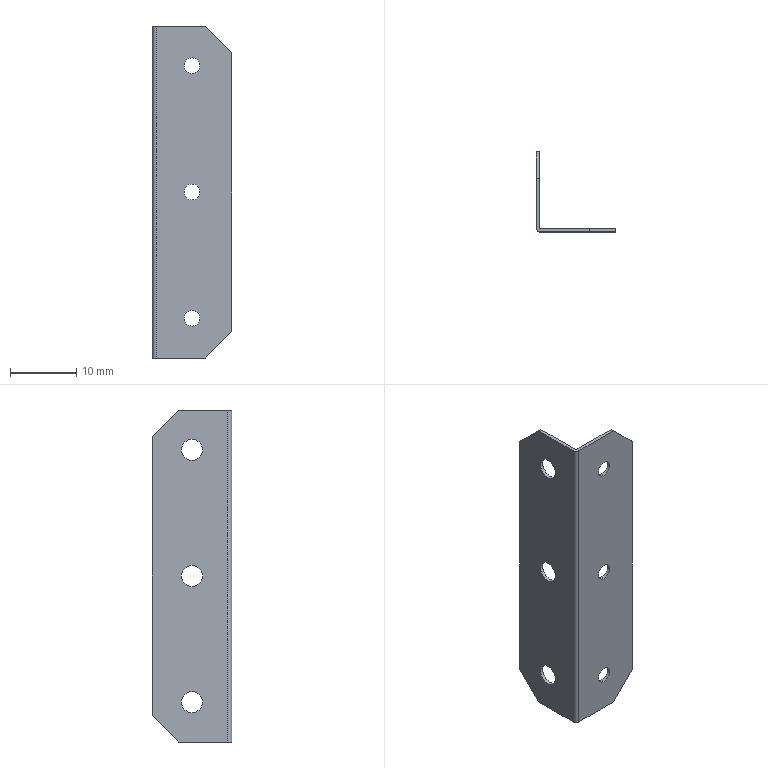Part | SolidWorks | features BaseBody 1 | 1 solid | 26 faces | box 12 x 12 x 50 mm | volume 548.895 mm3 | cylinder 14 | plane 12 | commonest cylinder face diameters 2.4 x6 3.2 x6 0.2 x1 1.2 x1
STEP:
#1=CARTESIAN_POINT('',(6.,0.5,23.8));
#2=VERTEX_POINT('',#1);
#3=CARTESIAN_POINT('',(6.,0.5,26.2));
#4=VERTEX_POINT('',#3);
#5=CARTESIAN_POINT('',(6.,0.5,25.));
#6=DIRECTION('',(0.,1.,0.));
#7=DIRECTION('',(0.,0.,-1.));
#8=AXIS2_PLACEMENT_3D('',#5,#6,#7);
#9=CIRCLE('',#8,1.2);
#10=EDGE_CURVE('',#2,#4,#9,.T.);
#11=ORIENTED_EDGE('',*,*,#10,.T.);
#12=CARTESIAN_POINT('',(6.,0.,26.2));
#13=VERTEX_POINT('',#12);
#14=CARTESIAN_POINT('',(6.,0.5,26.2));
#15=DIRECTION('',(0.,-1.,0.));
#16=VECTOR('',#15,1000.);
#17=LINE('',#14,#16);
#18=EDGE_CURVE('',#4,#13,#17,.T.);
#19=ORIENTED_EDGE('',*,*,#18,.T.);
#20=CARTESIAN_POINT('',(6.,0.,23.8));
#21=VERTEX_POINT('',#20);
#22=CARTESIAN_POINT('',(6.,0.,25.));
#23=DIRECTION('',(0.,-1.,0.));
#24=DIRECTION('',(0.,0.,-1.));
#25=AXIS2_PLACEMENT_3D('',#22,#23,#24);
#26=CIRCLE('',#25,1.2);
#27=EDGE_CURVE('',#13,#21,#26,.T.);
#28=ORIENTED_EDGE('',*,*,#27,.T.);
#29=CARTESIAN_POINT('',(6.,0.5,23.8));
#30=DIRECTION('',(0.,-1.,0.));
#31=VECTOR('',#30,1000.);
#32=LINE('',#29,#31);
#33=EDGE_CURVE('',#2,#21,#32,.T.);
#34=ORIENTED_EDGE('',*,*,#33,.F.);
#35=EDGE_LOOP('',(#11,#19,#28,#34));
#36=FACE_OUTER_BOUND('',#35,.T.);
#37=CARTESIAN_POINT('',(6.,0.5,25.));
#38=DIRECTION('',(0.,-1.,0.));
#39=DIRECTION('',(0.,0.,-1.));
#40=AXIS2_PLACEMENT_3D('',#37,#38,#39);
#41=CYLINDRICAL_SURFACE('',#40,1.2);
#42=ADVANCED_FACE('',(#36),#41,.F.);
#43=CARTESIAN_POINT('',(6.,0.5,42.8));
#44=VERTEX_POINT('',#43);
#45=CARTESIAN_POINT('',(6.,0.5,45.2));
#46=VERTEX_POINT('',#45);
#47=CARTESIAN_POINT('',(6.,0.5,44.));
#48=DIRECTION('',(0.,1.,0.));
#49=DIRECTION('',(0.,0.,-1.));
#50=AXIS2_PLACEMENT_3D('',#47,#48,#49);
#51=CIRCLE('',#50,1.2);
#52=EDGE_CURVE('',#44,#46,#51,.T.);
#53=ORIENTED_EDGE('',*,*,#52,.T.);
#54=CARTESIAN_POINT('',(6.,0.,45.2));
#55=VERTEX_POINT('',#54);
#56=CARTESIAN_POINT('',(6.,0.5,45.2));
#57=DIRECTION('',(0.,-1.,0.));
#58=VECTOR('',#57,1000.);
#59=LINE('',#56,#58);
#60=EDGE_CURVE('',#46,#55,#59,.T.);
#61=ORIENTED_EDGE('',*,*,#60,.T.);
#62=CARTESIAN_POINT('',(6.,0.,42.8));
#63=VERTEX_POINT('',#62);
#64=CARTESIAN_POINT('',(6.,0.,44.));
#65=DIRECTION('',(0.,-1.,0.));
#66=DIRECTION('',(0.,0.,-1.));
#67=AXIS2_PLACEMENT_3D('',#64,#65,#66);
#68=CIRCLE('',#67,1.2);
#69=EDGE_CURVE('',#55,#63,#68,.T.);
#70=ORIENTED_EDGE('',*,*,#69,.T.);
#71=CARTESIAN_POINT('',(6.,0.5,42.8));
#72=DIRECTION('',(0.,-1.,0.));
#73=VECTOR('',#72,1000.);
#74=LINE('',#71,#73);
#75=EDGE_CURVE('',#44,#63,#74,.T.);
#76=ORIENTED_EDGE('',*,*,#75,.F.);
#77=EDGE_LOOP('',(#53,#61,#70,#76));
#78=FACE_OUTER_BOUND('',#77,.T.);
#79=CARTESIAN_POINT('',(6.,0.5,44.));
#80=DIRECTION('',(0.,-1.,0.));
#81=DIRECTION('',(0.,0.,-1.));
#82=AXIS2_PLACEMENT_3D('',#79,#80,#81);
#83=CYLINDRICAL_SURFACE('',#82,1.2);
#84=ADVANCED_FACE('',(#78),#83,.F.);
#85=CARTESIAN_POINT('',(6.,0.5,4.8));
#86=VERTEX_POINT('',#85);
#87=CARTESIAN_POINT('',(6.,0.5,7.2));
#88=VERTEX_POINT('',#87);
#89=CARTESIAN_POINT('',(6.,0.5,6.));
#90=DIRECTION('',(0.,1.,0.));
#91=DIRECTION('',(0.,0.,-1.));
#92=AXIS2_PLACEMENT_3D('',#89,#90,#91);
#93=CIRCLE('',#92,1.2);
#94=EDGE_CURVE('',#86,#88,#93,.T.);
#95=ORIENTED_EDGE('',*,*,#94,.T.);
#96=CARTESIAN_POINT('',(6.,0.,7.2));
#97=VERTEX_POINT('',#96);
#98=CARTESIAN_POINT('',(6.,0.5,7.2));
#99=DIRECTION('',(0.,-1.,0.));
#100=VECTOR('',#99,1000.);
#101=LINE('',#98,#100);
#102=EDGE_CURVE('',#88,#97,#101,.T.);
#103=ORIENTED_EDGE('',*,*,#102,.T.);
#104=CARTESIAN_POINT('',(6.,0.,4.8));
#105=VERTEX_POINT('',#104);
#106=CARTESIAN_POINT('',(6.,0.,6.));
#107=DIRECTION('',(0.,-1.,0.));
#108=DIRECTION('',(0.,0.,-1.));
#109=AXIS2_PLACEMENT_3D('',#106,#107,#108);
#110=CIRCLE('',#109,1.2);
#111=EDGE_CURVE('',#97,#105,#110,.T.);
#112=ORIENTED_EDGE('',*,*,#111,.T.);
#113=CARTESIAN_POINT('',(6.,0.5,4.8));
#114=DIRECTION('',(0.,-1.,0.));
#115=VECTOR('',#114,1000.);
#116=LINE('',#113,#115);
#117=EDGE_CURVE('',#86,#105,#116,.T.);
#118=ORIENTED_EDGE('',*,*,#117,.F.);
#119=EDGE_LOOP('',(#95,#103,#112,#118));
#120=FACE_OUTER_BOUND('',#119,.T.);
#121=CARTESIAN_POINT('',(6.,0.5,6.));
#122=DIRECTION('',(0.,-1.,0.));
#123=DIRECTION('',(0.,0.,-1.));
#124=AXIS2_PLACEMENT_3D('',#121,#122,#123);
#125=CYLINDRICAL_SURFACE('',#124,1.2);
#126=ADVANCED_FACE('',(#120),#125,.F.);
#127=CARTESIAN_POINT('',(0.5,6.,7.6));
#128=VERTEX_POINT('',#127);
#129=CARTESIAN_POINT('',(0.5,6.,4.4));
#130=VERTEX_POINT('',#129);
#131=CARTESIAN_POINT('',(0.5,6.,6.));
#132=DIRECTION('',(1.,0.,0.));
#133=DIRECTION('',(0.,0.,1.));
#134=AXIS2_PLACEMENT_3D('',#131,#132,#133);
#135=CIRCLE('',#134,1.6);
#136=EDGE_CURVE('',#128,#130,#135,.T.);
#137=ORIENTED_EDGE('',*,*,#136,.T.);
#138=CARTESIAN_POINT('',(0.,6.,4.4));
#139=VERTEX_POINT('',#138);
#140=CARTESIAN_POINT('',(0.5,6.,4.4));
#141=DIRECTION('',(-1.,0.,0.));
#142=VECTOR('',#141,1000.);
#143=LINE('',#140,#142);
#144=EDGE_CURVE('',#130,#139,#143,.T.);
#145=ORIENTED_EDGE('',*,*,#144,.T.);
#146=CARTESIAN_POINT('',(0.,6.,7.6));
#147=VERTEX_POINT('',#146);
#148=CARTESIAN_POINT('',(0.,6.,6.));
#149=DIRECTION('',(-1.,0.,0.));
#150=DIRECTION('',(0.,0.,1.));
#151=AXIS2_PLACEMENT_3D('',#148,#149,#150);
#152=CIRCLE('',#151,1.6);
#153=EDGE_CURVE('',#139,#147,#152,.T.);
#154=ORIENTED_EDGE('',*,*,#153,.T.);
#155=CARTESIAN_POINT('',(0.5,6.,7.6));
#156=DIRECTION('',(-1.,0.,0.));
#157=VECTOR('',#156,1000.);
#158=LINE('',#155,#157);
#159=EDGE_CURVE('',#128,#147,#158,.T.);
#160=ORIENTED_EDGE('',*,*,#159,.F.);
#161=EDGE_LOOP('',(#137,#145,#154,#160));
#162=FACE_OUTER_BOUND('',#161,.T.);
#163=CARTESIAN_POINT('',(0.5,6.,6.));
#164=DIRECTION('',(-1.,0.,0.));
#165=DIRECTION('',(0.,0.,1.));
#166=AXIS2_PLACEMENT_3D('',#163,#164,#165);
#167=CYLINDRICAL_SURFACE('',#166,1.6);
#168=ADVANCED_FACE('',(#162),#167,.F.);
#169=CARTESIAN_POINT('',(0.5,6.,45.6));
#170=VERTEX_POINT('',#169);
#171=CARTESIAN_POINT('',(0.5,6.,42.4));
#172=VERTEX_POINT('',#171);
#173=CARTESIAN_POINT('',(0.5,6.,44.));
#174=DIRECTION('',(1.,0.,0.));
#175=DIRECTION('',(0.,0.,1.));
#176=AXIS2_PLACEMENT_3D('',#173,#174,#175);
#177=CIRCLE('',#176,1.6);
#178=EDGE_CURVE('',#170,#172,#177,.T.);
#179=ORIENTED_EDGE('',*,*,#178,.T.);
#180=CARTESIAN_POINT('',(0.,6.,42.4));
#181=VERTEX_POINT('',#180);
#182=CARTESIAN_POINT('',(0.5,6.,42.4));
#183=DIRECTION('',(-1.,0.,0.));
#184=VECTOR('',#183,1000.);
#185=LINE('',#182,#184);
#186=EDGE_CURVE('',#172,#181,#185,.T.);
#187=ORIENTED_EDGE('',*,*,#186,.T.);
#188=CARTESIAN_POINT('',(0.,6.,45.6));
#189=VERTEX_POINT('',#188);
#190=CARTESIAN_POINT('',(0.,6.,44.));
#191=DIRECTION('',(-1.,0.,0.));
#192=DIRECTION('',(0.,0.,1.));
#193=AXIS2_PLACEMENT_3D('',#190,#191,#192);
#194=CIRCLE('',#193,1.6);
#195=EDGE_CURVE('',#181,#189,#194,.T.);
#196=ORIENTED_EDGE('',*,*,#195,.T.);
#197=CARTESIAN_POINT('',(0.5,6.,45.6));
#198=DIRECTION('',(-1.,0.,0.));
#199=VECTOR('',#198,1000.);
#200=LINE('',#197,#199);
#201=EDGE_CURVE('',#170,#189,#200,.T.);
#202=ORIENTED_EDGE('',*,*,#201,.F.);
#203=EDGE_LOOP('',(#179,#187,#196,#202));
#204=FACE_OUTER_BOUND('',#203,.T.);
#205=CARTESIAN_POINT('',(0.5,6.,44.));
#206=DIRECTION('',(-1.,0.,0.));
#207=DIRECTION('',(0.,0.,1.));
#208=AXIS2_PLACEMENT_3D('',#205,#206,#207);
#209=CYLINDRICAL_SURFACE('',#208,1.6);
#210=ADVANCED_FACE('',(#204),#209,.F.);
#211=CARTESIAN_POINT('',(0.5,6.,26.6));
#212=VERTEX_POINT('',#211);
#213=CARTESIAN_POINT('',(0.5,6.,23.4));
#214=VERTEX_POINT('',#213);
#215=CARTESIAN_POINT('',(0.5,6.,25.));
#216=DIRECTION('',(1.,0.,0.));
#217=DIRECTION('',(0.,0.,1.));
#218=AXIS2_PLACEMENT_3D('',#215,#216,#217);
#219=CIRCLE('',#218,1.6);
#220=EDGE_CURVE('',#212,#214,#219,.T.);
#221=ORIENTED_EDGE('',*,*,#220,.T.);
#222=CARTESIAN_POINT('',(0.,6.,23.4));
#223=VERTEX_POINT('',#222);
#224=CARTESIAN_POINT('',(0.5,6.,23.4));
#225=DIRECTION('',(-1.,0.,0.));
#226=VECTOR('',#225,1000.);
#227=LINE('',#224,#226);
#228=EDGE_CURVE('',#214,#223,#227,.T.);
#229=ORIENTED_EDGE('',*,*,#228,.T.);
#230=CARTESIAN_POINT('',(0.,6.,26.6));
#231=VERTEX_POINT('',#230);
#232=CARTESIAN_POINT('',(0.,6.,25.));
#233=DIRECTION('',(-1.,0.,0.));
#234=DIRECTION('',(0.,0.,1.));
#235=AXIS2_PLACEMENT_3D('',#232,#233,#234);
#236=CIRCLE('',#235,1.6);
#237=EDGE_CURVE('',#223,#231,#236,.T.);
#238=ORIENTED_EDGE('',*,*,#237,.T.);
#239=CARTESIAN_POINT('',(0.5,6.,26.6));
#240=DIRECTION('',(-1.,0.,0.));
#241=VECTOR('',#240,1000.);
#242=LINE('',#239,#241);
#243=EDGE_CURVE('',#212,#231,#242,.T.);
#244=ORIENTED_EDGE('',*,*,#243,.F.);
#245=EDGE_LOOP('',(#221,#229,#238,#244));
#246=FACE_OUTER_BOUND('',#245,.T.);
#247=CARTESIAN_POINT('',(0.5,6.,25.));
#248=DIRECTION('',(-1.,0.,0.));
#249=DIRECTION('',(0.,0.,1.));
#250=AXIS2_PLACEMENT_3D('',#247,#248,#249);
#251=CYLINDRICAL_SURFACE('',#250,1.6);
#252=ADVANCED_FACE('',(#246),#251,.F.);
#253=ORIENTED_EDGE('',*,*,#18,.F.);
#254=CARTESIAN_POINT('',(6.,0.5,25.));
#255=DIRECTION('',(0.,1.,0.));
#256=DIRECTION('',(0.,0.,-1.));
#257=AXIS2_PLACEMENT_3D('',#254,#255,#256);
#258=CIRCLE('',#257,1.2);
#259=EDGE_CURVE('',#4,#2,#258,.T.);
#260=ORIENTED_EDGE('',*,*,#259,.T.);
#261=ORIENTED_EDGE('',*,*,#33,.T.);
#262=CARTESIAN_POINT('',(6.,0.,25.));
#263=DIRECTION('',(0.,-1.,0.));
#264=DIRECTION('',(0.,0.,-1.));
#265=AXIS2_PLACEMENT_3D('',#262,#263,#264);
#266=CIRCLE('',#265,1.2);
#267=EDGE_CURVE('',#21,#13,#266,.T.);
#268=ORIENTED_EDGE('',*,*,#267,.T.);
#269=EDGE_LOOP('',(#253,#260,#261,#268));
#270=FACE_OUTER_BOUND('',#269,.T.);
#271=CARTESIAN_POINT('',(6.,0.5,25.));
#272=DIRECTION('',(0.,-1.,0.));
#273=DIRECTION('',(0.,0.,-1.));
#274=AXIS2_PLACEMENT_3D('',#271,#272,#273);
#275=CYLINDRICAL_SURFACE('',#274,1.2);
#276=ADVANCED_FACE('',(#270),#275,.F.);
#277=CARTESIAN_POINT('',(6.,0.,44.));
#278=DIRECTION('',(0.,-1.,0.));
#279=DIRECTION('',(0.,0.,-1.));
#280=AXIS2_PLACEMENT_3D('',#277,#278,#279);
#281=CIRCLE('',#280,1.2);
#282=EDGE_CURVE('',#63,#55,#281,.T.);
#283=ORIENTED_EDGE('',*,*,#282,.F.);
#284=ORIENTED_EDGE('',*,*,#69,.F.);
#285=EDGE_LOOP('',(#283,#284));
#286=FACE_BOUND('',#285,.T.);
#287=CARTESIAN_POINT('',(6.,0.,6.));
#288=DIRECTION('',(0.,-1.,0.));
#289=DIRECTION('',(0.,0.,-1.));
#290=AXIS2_PLACEMENT_3D('',#287,#288,#289);
#291=CIRCLE('',#290,1.2);
#292=EDGE_CURVE('',#105,#97,#291,.T.);
#293=ORIENTED_EDGE('',*,*,#292,.F.);
#294=ORIENTED_EDGE('',*,*,#111,.F.);
#295=EDGE_LOOP('',(#293,#294));
#296=FACE_BOUND('',#295,.T.);
#297=ORIENTED_EDGE('',*,*,#267,.F.);
#298=ORIENTED_EDGE('',*,*,#27,.F.);
#299=EDGE_LOOP('',(#297,#298));
#300=FACE_BOUND('',#299,.T.);
#301=CARTESIAN_POINT('',(12.,0.,4.));
#302=VERTEX_POINT('',#301);
#303=CARTESIAN_POINT('',(8.,0.,0.));
#304=VERTEX_POINT('',#303);
#305=CARTESIAN_POINT('',(8.,0.,0.));
#306=DIRECTION('',(-0.7071,0.,-0.7071));
#307=VECTOR('',#306,1000.);
#308=LINE('',#305,#307);
#309=EDGE_CURVE('',#302,#304,#308,.T.);
#310=ORIENTED_EDGE('',*,*,#309,.F.);
#311=CARTESIAN_POINT('',(12.,0.,46.));
#312=VERTEX_POINT('',#311);
#313=CARTESIAN_POINT('',(12.,0.,25.));
#314=DIRECTION('',(0.,0.,-1.));
#315=VECTOR('',#314,1000.);
#316=LINE('',#313,#315);
#317=EDGE_CURVE('',#312,#302,#316,.T.);
#318=ORIENTED_EDGE('',*,*,#317,.F.);
#319=CARTESIAN_POINT('',(8.,0.,50.));
#320=VERTEX_POINT('',#319);
#321=CARTESIAN_POINT('',(8.,0.,50.));
#322=DIRECTION('',(0.7071,0.,-0.7071));
#323=VECTOR('',#322,1000.);
#324=LINE('',#321,#323);
#325=EDGE_CURVE('',#320,#312,#324,.T.);
#326=ORIENTED_EDGE('',*,*,#325,.F.);
#327=CARTESIAN_POINT('',(0.6,0.,50.));
#328=VERTEX_POINT('',#327);
#329=CARTESIAN_POINT('',(6.3,0.,50.));
#330=DIRECTION('',(1.,0.,0.));
#331=VECTOR('',#330,1000.);
#332=LINE('',#329,#331);
#333=EDGE_CURVE('',#328,#320,#332,.T.);
#334=ORIENTED_EDGE('',*,*,#333,.F.);
#335=CARTESIAN_POINT('',(0.6,0.,0.));
#336=VERTEX_POINT('',#335);
#337=CARTESIAN_POINT('',(0.6,0.,25.));
#338=DIRECTION('',(0.,0.,1.));
#339=VECTOR('',#338,1000.);
#340=LINE('',#337,#339);
#341=EDGE_CURVE('',#336,#328,#340,.T.);
#342=ORIENTED_EDGE('',*,*,#341,.F.);
#343=CARTESIAN_POINT('',(6.3,0.,0.));
#344=DIRECTION('',(-1.,0.,0.));
#345=VECTOR('',#344,1000.);
#346=LINE('',#343,#345);
#347=EDGE_CURVE('',#304,#336,#346,.T.);
#348=ORIENTED_EDGE('',*,*,#347,.F.);
#349=EDGE_LOOP('',(#310,#318,#326,#334,#342,#348));
#350=FACE_OUTER_BOUND('',#349,.T.);
#351=CARTESIAN_POINT('',(0.6,0.,0.));
#352=DIRECTION('',(0.,1.,0.));
#353=DIRECTION('',(0.,0.,1.));
#354=AXIS2_PLACEMENT_3D('',#351,#352,#353);
#355=PLANE('',#354);
#356=ADVANCED_FACE('',(#286,#296,#300,#350),#355,.F.);
#357=ORIENTED_EDGE('',*,*,#52,.F.);
#358=CARTESIAN_POINT('',(6.,0.5,44.));
#359=DIRECTION('',(0.,1.,0.));
#360=DIRECTION('',(0.,0.,-1.));
#361=AXIS2_PLACEMENT_3D('',#358,#359,#360);
#362=CIRCLE('',#361,1.2);
#363=EDGE_CURVE('',#46,#44,#362,.T.);
#364=ORIENTED_EDGE('',*,*,#363,.F.);
#365=EDGE_LOOP('',(#357,#364));
#366=FACE_BOUND('',#365,.T.);
#367=ORIENTED_EDGE('',*,*,#94,.F.);
#368=CARTESIAN_POINT('',(6.,0.5,6.));
#369=DIRECTION('',(0.,1.,0.));
#370=DIRECTION('',(0.,0.,-1.));
#371=AXIS2_PLACEMENT_3D('',#368,#369,#370);
#372=CIRCLE('',#371,1.2);
#373=EDGE_CURVE('',#88,#86,#372,.T.);
#374=ORIENTED_EDGE('',*,*,#373,.F.);
#375=EDGE_LOOP('',(#367,#374));
#376=FACE_BOUND('',#375,.T.);
#377=ORIENTED_EDGE('',*,*,#10,.F.);
#378=ORIENTED_EDGE('',*,*,#259,.F.);
#379=EDGE_LOOP('',(#377,#378));
#380=FACE_BOUND('',#379,.T.);
#381=CARTESIAN_POINT('',(8.,0.5,0.));
#382=VERTEX_POINT('',#381);
#383=CARTESIAN_POINT('',(12.,0.5,4.));
#384=VERTEX_POINT('',#383);
#385=CARTESIAN_POINT('',(8.,0.5,0.));
#386=DIRECTION('',(0.7071,0.,0.7071));
#387=VECTOR('',#386,1000.);
#388=LINE('',#385,#387);
#389=EDGE_CURVE('',#382,#384,#388,.T.);
#390=ORIENTED_EDGE('',*,*,#389,.F.);
#391=CARTESIAN_POINT('',(0.6,0.5,0.));
#392=VERTEX_POINT('',#391);
#393=CARTESIAN_POINT('',(6.3,0.5,0.));
#394=DIRECTION('',(1.,0.,0.));
#395=VECTOR('',#394,1000.);
#396=LINE('',#393,#395);
#397=EDGE_CURVE('',#392,#382,#396,.T.);
#398=ORIENTED_EDGE('',*,*,#397,.F.);
#399=CARTESIAN_POINT('',(0.6,0.5,50.));
#400=VERTEX_POINT('',#399);
#401=CARTESIAN_POINT('',(0.6,0.5,25.));
#402=DIRECTION('',(0.,0.,-1.));
#403=VECTOR('',#402,1000.);
#404=LINE('',#401,#403);
#405=EDGE_CURVE('',#400,#392,#404,.T.);
#406=ORIENTED_EDGE('',*,*,#405,.F.);
#407=CARTESIAN_POINT('',(8.,0.5,50.));
#408=VERTEX_POINT('',#407);
#409=CARTESIAN_POINT('',(6.3,0.5,50.));
#410=DIRECTION('',(-1.,0.,0.));
#411=VECTOR('',#410,1000.);
#412=LINE('',#409,#411);
#413=EDGE_CURVE('',#408,#400,#412,.T.);
#414=ORIENTED_EDGE('',*,*,#413,.F.);
#415=CARTESIAN_POINT('',(12.,0.5,46.));
#416=VERTEX_POINT('',#415);
#417=CARTESIAN_POINT('',(8.,0.5,50.));
#418=DIRECTION('',(-0.7071,0.,0.7071));
#419=VECTOR('',#418,1000.);
#420=LINE('',#417,#419);
#421=EDGE_CURVE('',#416,#408,#420,.T.);
#422=ORIENTED_EDGE('',*,*,#421,.F.);
#423=CARTESIAN_POINT('',(12.,0.5,25.));
#424=DIRECTION('',(0.,0.,1.));
#425=VECTOR('',#424,1000.);
#426=LINE('',#423,#425);
#427=EDGE_CURVE('',#384,#416,#426,.T.);
#428=ORIENTED_EDGE('',*,*,#427,.F.);
#429=EDGE_LOOP('',(#390,#398,#406,#414,#422,#428));
#430=FACE_OUTER_BOUND('',#429,.T.);
#431=CARTESIAN_POINT('',(0.6,0.5,50.));
#432=DIRECTION('',(0.,-1.,0.));
#433=DIRECTION('',(0.,0.,-1.));
#434=AXIS2_PLACEMENT_3D('',#431,#432,#433);
#435=PLANE('',#434);
#436=ADVANCED_FACE('',(#366,#376,#380,#430),#435,.F.);
#437=ORIENTED_EDGE('',*,*,#60,.F.);
#438=ORIENTED_EDGE('',*,*,#363,.T.);
#439=ORIENTED_EDGE('',*,*,#75,.T.);
#440=ORIENTED_EDGE('',*,*,#282,.T.);
#441=EDGE_LOOP('',(#437,#438,#439,#440));
#442=FACE_OUTER_BOUND('',#441,.T.);
#443=CARTESIAN_POINT('',(6.,0.5,44.));
#444=DIRECTION('',(0.,-1.,0.));
#445=DIRECTION('',(0.,0.,-1.));
#446=AXIS2_PLACEMENT_3D('',#443,#444,#445);
#447=CYLINDRICAL_SURFACE('',#446,1.2);
#448=ADVANCED_FACE('',(#442),#447,.F.);
#449=ORIENTED_EDGE('',*,*,#102,.F.);
#450=ORIENTED_EDGE('',*,*,#373,.T.);
#451=ORIENTED_EDGE('',*,*,#117,.T.);
#452=ORIENTED_EDGE('',*,*,#292,.T.);
#453=EDGE_LOOP('',(#449,#450,#451,#452));
#454=FACE_OUTER_BOUND('',#453,.T.);
#455=CARTESIAN_POINT('',(6.,0.5,6.));
#456=DIRECTION('',(0.,-1.,0.));
#457=DIRECTION('',(0.,0.,-1.));
#458=AXIS2_PLACEMENT_3D('',#455,#456,#457);
#459=CYLINDRICAL_SURFACE('',#458,1.2);
#460=ADVANCED_FACE('',(#454),#459,.F.);
#461=CARTESIAN_POINT('',(8.,4.,0.));
#462=DIRECTION('',(0.,1.,0.));
#463=VECTOR('',#462,1000.);
#464=LINE('',#461,#463);
#465=EDGE_CURVE('',#304,#382,#464,.T.);
#466=ORIENTED_EDGE('',*,*,#465,.F.);
#467=ORIENTED_EDGE('',*,*,#347,.T.);
#468=CARTESIAN_POINT('',(0.,0.6,0.));
#469=VERTEX_POINT('',#468);
#470=CARTESIAN_POINT('',(0.6,0.6,0.));
#471=DIRECTION('',(0.,0.,1.));
#472=DIRECTION('',(-1.,0.,0.));
#473=AXIS2_PLACEMENT_3D('',#470,#471,#472);
#474=CIRCLE('',#473,0.6);
#475=EDGE_CURVE('',#469,#336,#474,.T.);
#476=ORIENTED_EDGE('',*,*,#475,.F.);
#477=CARTESIAN_POINT('',(0.,8.,0.));
#478=VERTEX_POINT('',#477);
#479=CARTESIAN_POINT('',(0.,4.,0.));
#480=DIRECTION('',(0.,-1.,0.));
#481=VECTOR('',#480,1000.);
#482=LINE('',#479,#481);
#483=EDGE_CURVE('',#478,#469,#482,.T.);
#484=ORIENTED_EDGE('',*,*,#483,.F.);
#485=CARTESIAN_POINT('',(0.5,8.,0.));
#486=VERTEX_POINT('',#485);
#487=CARTESIAN_POINT('',(0.25,8.,0.));
#488=DIRECTION('',(1.,0.,0.));
#489=VECTOR('',#488,1000.);
#490=LINE('',#487,#489);
#491=EDGE_CURVE('',#478,#486,#490,.T.);
#492=ORIENTED_EDGE('',*,*,#491,.T.);
#493=CARTESIAN_POINT('',(0.5,0.6,0.));
#494=VERTEX_POINT('',#493);
#495=CARTESIAN_POINT('',(0.5,4.,0.));
#496=DIRECTION('',(0.,1.,0.));
#497=VECTOR('',#496,1000.);
#498=LINE('',#495,#497);
#499=EDGE_CURVE('',#494,#486,#498,.T.);
#500=ORIENTED_EDGE('',*,*,#499,.F.);
#501=CARTESIAN_POINT('',(0.6,0.6,0.));
#502=DIRECTION('',(0.,0.,-1.));
#503=DIRECTION('',(-1.,0.,0.));
#504=AXIS2_PLACEMENT_3D('',#501,#502,#503);
#505=CIRCLE('',#504,0.1);
#506=EDGE_CURVE('',#392,#494,#505,.T.);
#507=ORIENTED_EDGE('',*,*,#506,.F.);
#508=ORIENTED_EDGE('',*,*,#397,.T.);
#509=EDGE_LOOP('',(#466,#467,#476,#484,#492,#500,#507,#508));
#510=FACE_OUTER_BOUND('',#509,.T.);
#511=CARTESIAN_POINT('',(0.,0.,0.));
#512=DIRECTION('',(0.,0.,1.));
#513=DIRECTION('',(1.,0.,0.));
#514=AXIS2_PLACEMENT_3D('',#511,#512,#513);
#515=PLANE('',#514);
#516=ADVANCED_FACE('',(#510),#515,.F.);
#517=ORIENTED_EDGE('',*,*,#465,.T.);
#518=ORIENTED_EDGE('',*,*,#389,.T.);
#519=CARTESIAN_POINT('',(12.,0.25,4.));
#520=DIRECTION('',(0.,1.,0.));
#521=VECTOR('',#520,1000.);
#522=LINE('',#519,#521);
#523=EDGE_CURVE('',#302,#384,#522,.T.);
#524=ORIENTED_EDGE('',*,*,#523,.F.);
#525=ORIENTED_EDGE('',*,*,#309,.T.);
#526=EDGE_LOOP('',(#517,#518,#524,#525));
#527=FACE_OUTER_BOUND('',#526,.T.);
#528=CARTESIAN_POINT('',(8.,0.,0.));
#529=DIRECTION('',(-0.7071,0.,0.7071));
#530=DIRECTION('',(0.7071,0.,0.7071));
#531=AXIS2_PLACEMENT_3D('',#528,#529,#530);
#532=PLANE('',#531);
#533=ADVANCED_FACE('',(#527),#532,.F.);
#534=ORIENTED_EDGE('',*,*,#523,.T.);
#535=ORIENTED_EDGE('',*,*,#427,.T.);
#536=CARTESIAN_POINT('',(12.,0.25,46.));
#537=DIRECTION('',(0.,1.,0.));
#538=VECTOR('',#537,1000.);
#539=LINE('',#536,#538);
#540=EDGE_CURVE('',#312,#416,#539,.T.);
#541=ORIENTED_EDGE('',*,*,#540,.F.);
#542=ORIENTED_EDGE('',*,*,#317,.T.);
#543=EDGE_LOOP('',(#534,#535,#541,#542));
#544=FACE_OUTER_BOUND('',#543,.T.);
#545=CARTESIAN_POINT('',(12.,0.,4.));
#546=DIRECTION('',(-1.,0.,0.));
#547=DIRECTION('',(0.,0.,1.));
#548=AXIS2_PLACEMENT_3D('',#545,#546,#547);
#549=PLANE('',#548);
#550=ADVANCED_FACE('',(#544),#549,.F.);
#551=ORIENTED_EDGE('',*,*,#421,.T.);
#552=CARTESIAN_POINT('',(8.,0.25,50.));
#553=DIRECTION('',(0.,-1.,0.));
#554=VECTOR('',#553,1000.);
#555=LINE('',#552,#554);
#556=EDGE_CURVE('',#408,#320,#555,.T.);
#557=ORIENTED_EDGE('',*,*,#556,.T.);
#558=ORIENTED_EDGE('',*,*,#325,.T.);
#559=ORIENTED_EDGE('',*,*,#540,.T.);
#560=EDGE_LOOP('',(#551,#557,#558,#559));
#561=FACE_OUTER_BOUND('',#560,.T.);
#562=CARTESIAN_POINT('',(8.,0.,50.));
#563=DIRECTION('',(0.7071,0.,0.7071));
#564=DIRECTION('',(0.7071,0.,-0.7071));
#565=AXIS2_PLACEMENT_3D('',#562,#563,#564);
#566=PLANE('',#565);
#567=ADVANCED_FACE('',(#561),#566,.T.);
#568=CARTESIAN_POINT('',(0.,8.,50.));
#569=VERTEX_POINT('',#568);
#570=CARTESIAN_POINT('',(0.,0.6,50.));
#571=VERTEX_POINT('',#570);
#572=CARTESIAN_POINT('',(0.,4.,50.));
#573=DIRECTION('',(0.,-1.,0.));
#574=VECTOR('',#573,1000.);
#575=LINE('',#572,#574);
#576=EDGE_CURVE('',#569,#571,#575,.T.);
#577=ORIENTED_EDGE('',*,*,#576,.T.);
#578=CARTESIAN_POINT('',(0.6,0.6,50.));
#579=DIRECTION('',(0.,0.,1.));
#580=DIRECTION('',(-1.,0.,0.));
#581=AXIS2_PLACEMENT_3D('',#578,#579,#580);
#582=CIRCLE('',#581,0.6);
#583=EDGE_CURVE('',#571,#328,#582,.T.);
#584=ORIENTED_EDGE('',*,*,#583,.T.);
#585=ORIENTED_EDGE('',*,*,#333,.T.);
#586=ORIENTED_EDGE('',*,*,#556,.F.);
#587=ORIENTED_EDGE('',*,*,#413,.T.);
#588=CARTESIAN_POINT('',(0.5,0.6,50.));
#589=VERTEX_POINT('',#588);
#590=CARTESIAN_POINT('',(0.6,0.6,50.));
#591=DIRECTION('',(0.,0.,-1.));
#592=DIRECTION('',(-1.,0.,0.));
#593=AXIS2_PLACEMENT_3D('',#590,#591,#592);
#594=CIRCLE('',#593,0.1);
#595=EDGE_CURVE('',#400,#589,#594,.T.);
#596=ORIENTED_EDGE('',*,*,#595,.T.);
#597=CARTESIAN_POINT('',(0.5,8.,50.));
#598=VERTEX_POINT('',#597);
#599=CARTESIAN_POINT('',(0.5,4.,50.));
#600=DIRECTION('',(0.,1.,0.));
#601=VECTOR('',#600,1000.);
#602=LINE('',#599,#601);
#603=EDGE_CURVE('',#589,#598,#602,.T.);
#604=ORIENTED_EDGE('',*,*,#603,.T.);
#605=CARTESIAN_POINT('',(0.25,8.,50.));
#606=DIRECTION('',(1.,0.,0.));
#607=VECTOR('',#606,1000.);
#608=LINE('',#605,#607);
#609=EDGE_CURVE('',#569,#598,#608,.T.);
#610=ORIENTED_EDGE('',*,*,#609,.F.);
#611=EDGE_LOOP('',(#577,#584,#585,#586,#587,#596,#604,#610));
#612=FACE_OUTER_BOUND('',#611,.T.);
#613=CARTESIAN_POINT('',(0.,0.,50.));
#614=DIRECTION('',(0.,0.,1.));
#615=DIRECTION('',(1.,0.,0.));
#616=AXIS2_PLACEMENT_3D('',#613,#614,#615);
#617=PLANE('',#616);
#618=ADVANCED_FACE('',(#612),#617,.T.);
#619=ORIENTED_EDGE('',*,*,#341,.T.);
#620=ORIENTED_EDGE('',*,*,#583,.F.);
#621=CARTESIAN_POINT('',(0.,0.6,25.));
#622=DIRECTION('',(0.,0.,1.));
#623=VECTOR('',#622,1000.);
#624=LINE('',#621,#623);
#625=EDGE_CURVE('',#469,#571,#624,.T.);
#626=ORIENTED_EDGE('',*,*,#625,.F.);
#627=ORIENTED_EDGE('',*,*,#475,.T.);
#628=EDGE_LOOP('',(#619,#620,#626,#627));
#629=FACE_OUTER_BOUND('',#628,.T.);
#630=CARTESIAN_POINT('',(0.6,0.6,50.));
#631=DIRECTION('',(0.,0.,-1.));
#632=DIRECTION('',(-1.,0.,0.));
#633=AXIS2_PLACEMENT_3D('',#630,#631,#632);
#634=CYLINDRICAL_SURFACE('',#633,0.6);
#635=ADVANCED_FACE('',(#629),#634,.T.);
#636=ORIENTED_EDGE('',*,*,#595,.F.);
#637=ORIENTED_EDGE('',*,*,#405,.T.);
#638=ORIENTED_EDGE('',*,*,#506,.T.);
#639=CARTESIAN_POINT('',(0.5,0.6,25.));
#640=DIRECTION('',(0.,0.,1.));
#641=VECTOR('',#640,1000.);
#642=LINE('',#639,#641);
#643=EDGE_CURVE('',#494,#589,#642,.T.);
#644=ORIENTED_EDGE('',*,*,#643,.T.);
#645=EDGE_LOOP('',(#636,#637,#638,#644));
#646=FACE_OUTER_BOUND('',#645,.T.);
#647=CARTESIAN_POINT('',(0.6,0.6,50.));
#648=DIRECTION('',(0.,0.,-1.));
#649=DIRECTION('',(-1.,0.,0.));
#650=AXIS2_PLACEMENT_3D('',#647,#648,#649);
#651=CYLINDRICAL_SURFACE('',#650,0.1);
#652=ADVANCED_FACE('',(#646),#651,.F.);
#653=CARTESIAN_POINT('',(0.,6.,6.));
#654=DIRECTION('',(-1.,0.,0.));
#655=DIRECTION('',(0.,0.,1.));
#656=AXIS2_PLACEMENT_3D('',#653,#654,#655);
#657=CIRCLE('',#656,1.6);
#658=EDGE_CURVE('',#147,#139,#657,.T.);
#659=ORIENTED_EDGE('',*,*,#658,.F.);
#660=ORIENTED_EDGE('',*,*,#153,.F.);
#661=EDGE_LOOP('',(#659,#660));
#662=FACE_BOUND('',#661,.T.);
#663=CARTESIAN_POINT('',(0.,6.,44.));
#664=DIRECTION('',(-1.,0.,0.));
#665=DIRECTION('',(0.,0.,1.));
#666=AXIS2_PLACEMENT_3D('',#663,#664,#665);
#667=CIRCLE('',#666,1.6);
#668=EDGE_CURVE('',#189,#181,#667,.T.);
#669=ORIENTED_EDGE('',*,*,#668,.F.);
#670=ORIENTED_EDGE('',*,*,#195,.F.);
#671=EDGE_LOOP('',(#669,#670));
#672=FACE_BOUND('',#671,.T.);
#673=CARTESIAN_POINT('',(0.,6.,25.));
#674=DIRECTION('',(-1.,0.,0.));
#675=DIRECTION('',(0.,0.,1.));
#676=AXIS2_PLACEMENT_3D('',#673,#674,#675);
#677=CIRCLE('',#676,1.6);
#678=EDGE_CURVE('',#231,#223,#677,.T.);
#679=ORIENTED_EDGE('',*,*,#678,.F.);
#680=ORIENTED_EDGE('',*,*,#237,.F.);
#681=EDGE_LOOP('',(#679,#680));
#682=FACE_BOUND('',#681,.T.);
#683=CARTESIAN_POINT('',(0.,12.,4.));
#684=VERTEX_POINT('',#683);
#685=CARTESIAN_POINT('',(0.,12.,4.));
#686=DIRECTION('',(0.,0.7071,0.7071));
#687=VECTOR('',#686,1000.);
#688=LINE('',#685,#687);
#689=EDGE_CURVE('',#478,#684,#688,.T.);
#690=ORIENTED_EDGE('',*,*,#689,.F.);
#691=ORIENTED_EDGE('',*,*,#483,.T.);
#692=ORIENTED_EDGE('',*,*,#625,.T.);
#693=ORIENTED_EDGE('',*,*,#576,.F.);
#694=CARTESIAN_POINT('',(0.,12.,46.));
#695=VERTEX_POINT('',#694);
#696=CARTESIAN_POINT('',(0.,12.,46.));
#697=DIRECTION('',(0.,-0.7071,0.7071));
#698=VECTOR('',#697,1000.);
#699=LINE('',#696,#698);
#700=EDGE_CURVE('',#695,#569,#699,.T.);
#701=ORIENTED_EDGE('',*,*,#700,.F.);
#702=CARTESIAN_POINT('',(0.,12.,25.));
#703=DIRECTION('',(0.,0.,1.));
#704=VECTOR('',#703,1000.);
#705=LINE('',#702,#704);
#706=EDGE_CURVE('',#684,#695,#705,.T.);
#707=ORIENTED_EDGE('',*,*,#706,.F.);
#708=EDGE_LOOP('',(#690,#691,#692,#693,#701,#707));
#709=FACE_OUTER_BOUND('',#708,.T.);
#710=CARTESIAN_POINT('',(0.,0.6,0.));
#711=DIRECTION('',(1.,0.,0.));
#712=DIRECTION('',(0.,1.,0.));
#713=AXIS2_PLACEMENT_3D('',#710,#711,#712);
#714=PLANE('',#713);
#715=ADVANCED_FACE('',(#662,#672,#682,#709),#714,.F.);
#716=ORIENTED_EDGE('',*,*,#136,.F.);
#717=CARTESIAN_POINT('',(0.5,6.,6.));
#718=DIRECTION('',(1.,0.,0.));
#719=DIRECTION('',(0.,0.,1.));
#720=AXIS2_PLACEMENT_3D('',#717,#718,#719);
#721=CIRCLE('',#720,1.6);
#722=EDGE_CURVE('',#130,#128,#721,.T.);
#723=ORIENTED_EDGE('',*,*,#722,.F.);
#724=EDGE_LOOP('',(#716,#723));
#725=FACE_BOUND('',#724,.T.);
#726=ORIENTED_EDGE('',*,*,#178,.F.);
#727=CARTESIAN_POINT('',(0.5,6.,44.));
#728=DIRECTION('',(1.,0.,0.));
#729=DIRECTION('',(0.,0.,1.));
#730=AXIS2_PLACEMENT_3D('',#727,#728,#729);
#731=CIRCLE('',#730,1.6);
#732=EDGE_CURVE('',#172,#170,#731,.T.);
#733=ORIENTED_EDGE('',*,*,#732,.F.);
#734=EDGE_LOOP('',(#726,#733));
#735=FACE_BOUND('',#734,.T.);
#736=ORIENTED_EDGE('',*,*,#220,.F.);
#737=CARTESIAN_POINT('',(0.5,6.,25.));
#738=DIRECTION('',(1.,0.,0.));
#739=DIRECTION('',(0.,0.,1.));
#740=AXIS2_PLACEMENT_3D('',#737,#738,#739);
#741=CIRCLE('',#740,1.6);
#742=EDGE_CURVE('',#214,#212,#741,.T.);
#743=ORIENTED_EDGE('',*,*,#742,.F.);
#744=EDGE_LOOP('',(#736,#743));
#745=FACE_BOUND('',#744,.T.);
#746=CARTESIAN_POINT('',(0.5,12.,4.));
#747=VERTEX_POINT('',#746);
#748=CARTESIAN_POINT('',(0.5,12.,4.));
#749=DIRECTION('',(0.,-0.7071,-0.7071));
#750=VECTOR('',#749,1000.);
#751=LINE('',#748,#750);
#752=EDGE_CURVE('',#747,#486,#751,.T.);
#753=ORIENTED_EDGE('',*,*,#752,.F.);
#754=CARTESIAN_POINT('',(0.5,12.,46.));
#755=VERTEX_POINT('',#754);
#756=CARTESIAN_POINT('',(0.5,12.,25.));
#757=DIRECTION('',(0.,0.,-1.));
#758=VECTOR('',#757,1000.);
#759=LINE('',#756,#758);
#760=EDGE_CURVE('',#755,#747,#759,.T.);
#761=ORIENTED_EDGE('',*,*,#760,.F.);
#762=CARTESIAN_POINT('',(0.5,12.,46.));
#763=DIRECTION('',(0.,0.7071,-0.7071));
#764=VECTOR('',#763,1000.);
#765=LINE('',#762,#764);
#766=EDGE_CURVE('',#598,#755,#765,.T.);
#767=ORIENTED_EDGE('',*,*,#766,.F.);
#768=ORIENTED_EDGE('',*,*,#603,.F.);
#769=ORIENTED_EDGE('',*,*,#643,.F.);
#770=ORIENTED_EDGE('',*,*,#499,.T.);
#771=EDGE_LOOP('',(#753,#761,#767,#768,#769,#770));
#772=FACE_OUTER_BOUND('',#771,.T.);
#773=CARTESIAN_POINT('',(0.5,0.6,0.));
#774=DIRECTION('',(-1.,0.,0.));
#775=DIRECTION('',(0.,0.,1.));
#776=AXIS2_PLACEMENT_3D('',#773,#774,#775);
#777=PLANE('',#776);
#778=ADVANCED_FACE('',(#725,#735,#745,#772),#777,.F.);
#779=ORIENTED_EDGE('',*,*,#144,.F.);
#780=ORIENTED_EDGE('',*,*,#722,.T.);
#781=ORIENTED_EDGE('',*,*,#159,.T.);
#782=ORIENTED_EDGE('',*,*,#658,.T.);
#783=EDGE_LOOP('',(#779,#780,#781,#782));
#784=FACE_OUTER_BOUND('',#783,.T.);
#785=CARTESIAN_POINT('',(0.5,6.,6.));
#786=DIRECTION('',(-1.,0.,0.));
#787=DIRECTION('',(0.,0.,1.));
#788=AXIS2_PLACEMENT_3D('',#785,#786,#787);
#789=CYLINDRICAL_SURFACE('',#788,1.6);
#790=ADVANCED_FACE('',(#784),#789,.F.);
#791=ORIENTED_EDGE('',*,*,#186,.F.);
#792=ORIENTED_EDGE('',*,*,#732,.T.);
#793=ORIENTED_EDGE('',*,*,#201,.T.);
#794=ORIENTED_EDGE('',*,*,#668,.T.);
#795=EDGE_LOOP('',(#791,#792,#793,#794));
#796=FACE_OUTER_BOUND('',#795,.T.);
#797=CARTESIAN_POINT('',(0.5,6.,44.));
#798=DIRECTION('',(-1.,0.,0.));
#799=DIRECTION('',(0.,0.,1.));
#800=AXIS2_PLACEMENT_3D('',#797,#798,#799);
#801=CYLINDRICAL_SURFACE('',#800,1.6);
#802=ADVANCED_FACE('',(#796),#801,.F.);
#803=ORIENTED_EDGE('',*,*,#228,.F.);
#804=ORIENTED_EDGE('',*,*,#742,.T.);
#805=ORIENTED_EDGE('',*,*,#243,.T.);
#806=ORIENTED_EDGE('',*,*,#678,.T.);
#807=EDGE_LOOP('',(#803,#804,#805,#806));
#808=FACE_OUTER_BOUND('',#807,.T.);
#809=CARTESIAN_POINT('',(0.5,6.,25.));
#810=DIRECTION('',(-1.,0.,0.));
#811=DIRECTION('',(0.,0.,1.));
#812=AXIS2_PLACEMENT_3D('',#809,#810,#811);
#813=CYLINDRICAL_SURFACE('',#812,1.6);
#814=ADVANCED_FACE('',(#808),#813,.F.);
#815=CARTESIAN_POINT('',(0.25,12.,4.));
#816=DIRECTION('',(1.,0.,0.));
#817=VECTOR('',#816,1000.);
#818=LINE('',#815,#817);
#819=EDGE_CURVE('',#684,#747,#818,.T.);
#820=ORIENTED_EDGE('',*,*,#819,.F.);
#821=ORIENTED_EDGE('',*,*,#706,.T.);
#822=CARTESIAN_POINT('',(0.25,12.,46.));
#823=DIRECTION('',(-1.,0.,0.));
#824=VECTOR('',#823,1000.);
#825=LINE('',#822,#824);
#826=EDGE_CURVE('',#755,#695,#825,.T.);
#827=ORIENTED_EDGE('',*,*,#826,.F.);
#828=ORIENTED_EDGE('',*,*,#760,.T.);
#829=EDGE_LOOP('',(#820,#821,#827,#828));
#830=FACE_OUTER_BOUND('',#829,.T.);
#831=CARTESIAN_POINT('',(0.,12.,46.));
#832=DIRECTION('',(0.,-1.,0.));
#833=DIRECTION('',(0.,0.,-1.));
#834=AXIS2_PLACEMENT_3D('',#831,#832,#833);
#835=PLANE('',#834);
#836=ADVANCED_FACE('',(#830),#835,.F.);
#837=ORIENTED_EDGE('',*,*,#491,.F.);
#838=ORIENTED_EDGE('',*,*,#689,.T.);
#839=ORIENTED_EDGE('',*,*,#819,.T.);
#840=ORIENTED_EDGE('',*,*,#752,.T.);
#841=EDGE_LOOP('',(#837,#838,#839,#840));
#842=FACE_OUTER_BOUND('',#841,.T.);
#843=CARTESIAN_POINT('',(0.,12.,4.));
#844=DIRECTION('',(0.,-0.7071,0.7071));
#845=DIRECTION('',(0.,-0.7071,-0.7071));
#846=AXIS2_PLACEMENT_3D('',#843,#844,#845);
#847=PLANE('',#846);
#848=ADVANCED_FACE('',(#842),#847,.F.);
#849=ORIENTED_EDGE('',*,*,#700,.T.);
#850=ORIENTED_EDGE('',*,*,#609,.T.);
#851=ORIENTED_EDGE('',*,*,#766,.T.);
#852=ORIENTED_EDGE('',*,*,#826,.T.);
#853=EDGE_LOOP('',(#849,#850,#851,#852));
#854=FACE_OUTER_BOUND('',#853,.T.);
#855=CARTESIAN_POINT('',(0.,12.,46.));
#856=DIRECTION('',(0.,0.7071,0.7071));
#857=DIRECTION('',(0.,-0.7071,0.7071));
#858=AXIS2_PLACEMENT_3D('',#855,#856,#857);
#859=PLANE('',#858);
#860=ADVANCED_FACE('',(#854),#859,.T.);
#861=CLOSED_SHELL('',(#42,#84,#126,#168,#210,#252,#276,#356,#436,#448,#460,#516,#533,#550,#567,#618,#635,#652,#715,#778,#790,#802,#814,#836,#848,#860));
#862=MANIFOLD_SOLID_BREP('',#861);
#863=CARTESIAN_POINT('',(0.,0.,0.));
#864=DIRECTION('',(0.,0.,1.));
#865=DIRECTION('',(1.,0.,0.));
#866=AXIS2_PLACEMENT_3D('',#863,#864,#865);
#867=(LENGTH_UNIT()NAMED_UNIT(*)SI_UNIT(.MILLI.,.METRE.));
#868=UNCERTAINTY_MEASURE_WITH_UNIT(LENGTH_MEASURE(0.00001),#867,'','');
#869=(NAMED_UNIT(*)PLANE_ANGLE_UNIT()SI_UNIT($,.RADIAN.));
#870=(NAMED_UNIT(*)SI_UNIT($,.STERADIAN.)SOLID_ANGLE_UNIT());
#871=(GEOMETRIC_REPRESENTATION_CONTEXT(3)GLOBAL_UNCERTAINTY_ASSIGNED_CONTEXT((#868))GLOBAL_UNIT_ASSIGNED_CONTEXT((#867,#869,#870))REPRESENTATION_CONTEXT('',''));
#872=ADVANCED_BREP_SHAPE_REPRESENTATION('',(#862,#866),#871);